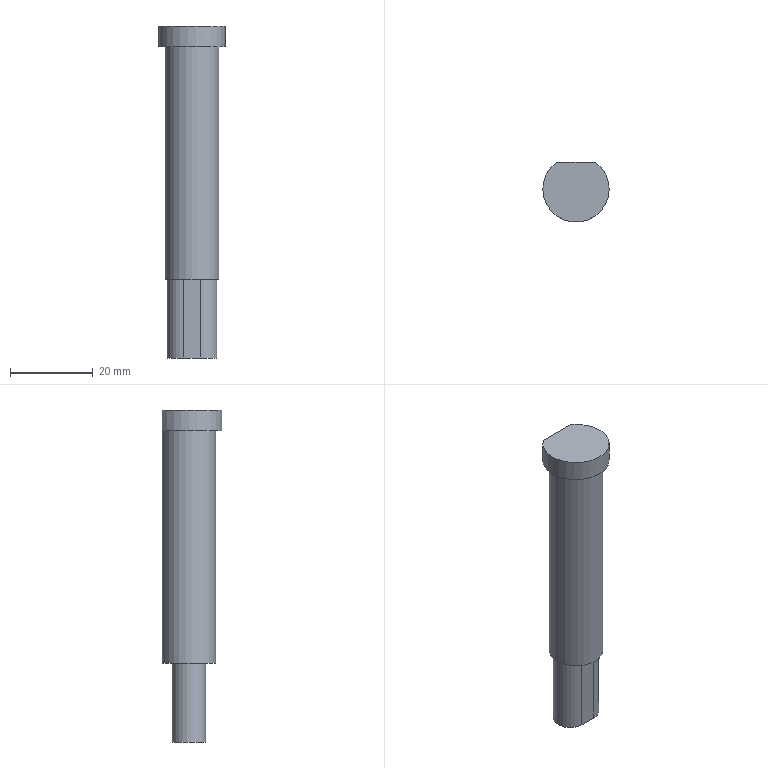Part | NX | features solid 2 | 1 solid | 11 faces | box 16 x 14.5 x 80 mm | volume 9985 mm3 | plane 7 | cylinder 4 | commonest cylinder face diameters 8.1 x2 13 x1 16 x1
STEP:
#1=CARTESIAN_POINT('',(-1262.413,378.428,72.));
#2=VERTEX_POINT('',#1);
#3=CARTESIAN_POINT('',(-1262.413,384.928,72.));
#4=DIRECTION('',(0.,0.,1.));
#5=DIRECTION('',(0.,-1.,0.));
#6=AXIS2_PLACEMENT_3D('',#3,#4,#5);
#7=CIRCLE('',#6,6.5);
#8=EDGE_CURVE('',#2,#2,#7,.T.);
#9=ORIENTED_EDGE('',*,*,#8,.F.);
#10=EDGE_LOOP('',(#9));
#11=FACE_BOUND('',#10,.T.);
#12=CARTESIAN_POINT('',(-1260.413,380.878,72.));
#13=VERTEX_POINT('',#12);
#14=CARTESIAN_POINT('',(-1264.413,380.878,72.));
#15=VERTEX_POINT('',#14);
#16=CARTESIAN_POINT('',(-1262.413,380.878,72.));
#17=DIRECTION('',(-1.,0.,0.));
#18=VECTOR('',#17,1000.);
#19=LINE('',#16,#18);
#20=EDGE_CURVE('',#13,#15,#19,.T.);
#21=ORIENTED_EDGE('',*,*,#20,.F.);
#22=CARTESIAN_POINT('',(-1260.413,388.978,72.));
#23=VERTEX_POINT('',#22);
#24=CARTESIAN_POINT('',(-1260.413,384.928,72.));
#25=DIRECTION('',(0.,0.,1.));
#26=DIRECTION('',(0.,-1.,0.));
#27=AXIS2_PLACEMENT_3D('',#24,#25,#26);
#28=CIRCLE('',#27,4.05);
#29=EDGE_CURVE('',#13,#23,#28,.T.);
#30=ORIENTED_EDGE('',*,*,#29,.T.);
#31=CARTESIAN_POINT('',(-1264.413,388.978,72.));
#32=VERTEX_POINT('',#31);
#33=CARTESIAN_POINT('',(-1262.413,388.978,72.));
#34=DIRECTION('',(-1.,0.,0.));
#35=VECTOR('',#34,1000.);
#36=LINE('',#33,#35);
#37=EDGE_CURVE('',#23,#32,#36,.T.);
#38=ORIENTED_EDGE('',*,*,#37,.T.);
#39=CARTESIAN_POINT('',(-1264.413,384.928,72.));
#40=DIRECTION('',(0.,0.,1.));
#41=DIRECTION('',(0.,-1.,0.));
#42=AXIS2_PLACEMENT_3D('',#39,#40,#41);
#43=CIRCLE('',#42,4.05);
#44=EDGE_CURVE('',#32,#15,#43,.T.);
#45=ORIENTED_EDGE('',*,*,#44,.T.);
#46=EDGE_LOOP('',(#21,#30,#38,#45));
#47=FACE_BOUND('',#46,.T.);
#48=CARTESIAN_POINT('',(-1262.413,384.928,72.));
#49=DIRECTION('',(0.,0.,1.));
#50=DIRECTION('',(0.,-1.,0.));
#51=AXIS2_PLACEMENT_3D('',#48,#49,#50);
#52=PLANE('',#51);
#53=ADVANCED_FACE('',(#11,#47),#52,.F.);
#54=ORIENTED_EDGE('',*,*,#8,.T.);
#55=EDGE_LOOP('',(#54));
#56=FACE_BOUND('',#55,.T.);
#57=CARTESIAN_POINT('',(-1262.413,391.428,128.));
#58=VERTEX_POINT('',#57);
#59=CARTESIAN_POINT('',(-1262.413,384.928,128.));
#60=DIRECTION('',(0.,0.,1.));
#61=DIRECTION('',(0.,-1.,0.));
#62=AXIS2_PLACEMENT_3D('',#59,#60,#61);
#63=CIRCLE('',#62,6.5);
#64=EDGE_CURVE('',#58,#58,#63,.T.);
#65=ORIENTED_EDGE('',*,*,#64,.F.);
#66=EDGE_LOOP('',(#65));
#67=FACE_BOUND('',#66,.T.);
#68=CARTESIAN_POINT('',(-1262.413,384.928,133.));
#69=DIRECTION('',(0.,0.,-1.));
#70=DIRECTION('',(0.,1.,0.));
#71=AXIS2_PLACEMENT_3D('',#68,#69,#70);
#72=CYLINDRICAL_SURFACE('',#71,6.5);
#73=ADVANCED_FACE('',(#56,#67),#72,.T.);
#74=CARTESIAN_POINT('',(-1267.077,391.428,128.));
#75=VERTEX_POINT('',#74);
#76=CARTESIAN_POINT('',(-1257.75,391.428,128.));
#77=VERTEX_POINT('',#76);
#78=CARTESIAN_POINT('',(-1262.413,384.928,128.));
#79=DIRECTION('',(0.,0.,1.));
#80=DIRECTION('',(0.,-1.,0.));
#81=AXIS2_PLACEMENT_3D('',#78,#79,#80);
#82=CIRCLE('',#81,8.);
#83=EDGE_CURVE('',#75,#77,#82,.T.);
#84=ORIENTED_EDGE('',*,*,#83,.F.);
#85=CARTESIAN_POINT('',(-1262.413,391.428,128.));
#86=DIRECTION('',(1.,0.,0.));
#87=VECTOR('',#86,1000.);
#88=LINE('',#85,#87);
#89=EDGE_CURVE('',#75,#58,#88,.T.);
#90=ORIENTED_EDGE('',*,*,#89,.T.);
#91=ORIENTED_EDGE('',*,*,#64,.T.);
#92=CARTESIAN_POINT('',(-1262.413,391.428,128.));
#93=DIRECTION('',(1.,0.,0.));
#94=VECTOR('',#93,1000.);
#95=LINE('',#92,#94);
#96=EDGE_CURVE('',#58,#77,#95,.T.);
#97=ORIENTED_EDGE('',*,*,#96,.T.);
#98=EDGE_LOOP('',(#84,#90,#91,#97));
#99=FACE_BOUND('',#98,.T.);
#100=CARTESIAN_POINT('',(-1262.413,384.928,128.));
#101=DIRECTION('',(0.,0.,1.));
#102=DIRECTION('',(0.,-1.,0.));
#103=AXIS2_PLACEMENT_3D('',#100,#101,#102);
#104=PLANE('',#103);
#105=ADVANCED_FACE('',(#99),#104,.F.);
#106=CARTESIAN_POINT('',(-1257.75,391.428,133.));
#107=VERTEX_POINT('',#106);
#108=CARTESIAN_POINT('',(-1257.75,391.428,137.));
#109=DIRECTION('',(0.,0.,-1.));
#110=VECTOR('',#109,1000.);
#111=LINE('',#108,#110);
#112=EDGE_CURVE('',#107,#77,#111,.T.);
#113=ORIENTED_EDGE('',*,*,#112,.F.);
#114=CARTESIAN_POINT('',(-1267.077,391.428,133.));
#115=VERTEX_POINT('',#114);
#116=CARTESIAN_POINT('',(-1262.413,384.928,133.));
#117=DIRECTION('',(0.,0.,1.));
#118=DIRECTION('',(0.,-1.,0.));
#119=AXIS2_PLACEMENT_3D('',#116,#117,#118);
#120=CIRCLE('',#119,8.);
#121=EDGE_CURVE('',#115,#107,#120,.T.);
#122=ORIENTED_EDGE('',*,*,#121,.F.);
#123=CARTESIAN_POINT('',(-1267.077,391.428,137.));
#124=DIRECTION('',(0.,0.,-1.));
#125=VECTOR('',#124,1000.);
#126=LINE('',#123,#125);
#127=EDGE_CURVE('',#75,#115,#126,.F.);
#128=ORIENTED_EDGE('',*,*,#127,.F.);
#129=ORIENTED_EDGE('',*,*,#83,.T.);
#130=EDGE_LOOP('',(#113,#122,#128,#129));
#131=FACE_BOUND('',#130,.T.);
#132=CARTESIAN_POINT('',(-1262.413,384.928,128.));
#133=DIRECTION('',(0.,0.,1.));
#134=DIRECTION('',(0.,-1.,0.));
#135=AXIS2_PLACEMENT_3D('',#132,#133,#134);
#136=CYLINDRICAL_SURFACE('',#135,8.);
#137=ADVANCED_FACE('',(#131),#136,.T.);
#138=CARTESIAN_POINT('',(-1262.413,391.428,133.));
#139=DIRECTION('',(1.,0.,0.));
#140=VECTOR('',#139,1000.);
#141=LINE('',#138,#140);
#142=EDGE_CURVE('',#115,#107,#141,.T.);
#143=ORIENTED_EDGE('',*,*,#142,.F.);
#144=ORIENTED_EDGE('',*,*,#121,.T.);
#145=EDGE_LOOP('',(#143,#144));
#146=FACE_BOUND('',#145,.T.);
#147=CARTESIAN_POINT('',(-1262.413,384.928,133.));
#148=DIRECTION('',(0.,0.,1.));
#149=DIRECTION('',(0.,-1.,0.));
#150=AXIS2_PLACEMENT_3D('',#147,#148,#149);
#151=PLANE('',#150);
#152=ADVANCED_FACE('',(#146),#151,.T.);
#153=ORIENTED_EDGE('',*,*,#127,.T.);
#154=ORIENTED_EDGE('',*,*,#142,.T.);
#155=ORIENTED_EDGE('',*,*,#112,.T.);
#156=ORIENTED_EDGE('',*,*,#96,.F.);
#157=ORIENTED_EDGE('',*,*,#89,.F.);
#158=EDGE_LOOP('',(#153,#154,#155,#156,#157));
#159=FACE_BOUND('',#158,.T.);
#160=CARTESIAN_POINT('',(-1257.75,391.428,137.));
#161=DIRECTION('',(0.,-1.,0.));
#162=DIRECTION('',(0.,0.,-1.));
#163=AXIS2_PLACEMENT_3D('',#160,#161,#162);
#164=PLANE('',#163);
#165=ADVANCED_FACE('',(#159),#164,.F.);
#166=CARTESIAN_POINT('',(-1260.413,380.878,53.));
#167=VERTEX_POINT('',#166);
#168=CARTESIAN_POINT('',(-1260.413,380.878,53.));
#169=DIRECTION('',(0.,0.,1.));
#170=VECTOR('',#169,1000.);
#171=LINE('',#168,#170);
#172=EDGE_CURVE('',#167,#13,#171,.T.);
#173=ORIENTED_EDGE('',*,*,#172,.T.);
#174=ORIENTED_EDGE('',*,*,#20,.T.);
#175=CARTESIAN_POINT('',(-1264.413,380.878,53.));
#176=VERTEX_POINT('',#175);
#177=CARTESIAN_POINT('',(-1264.413,380.878,53.));
#178=DIRECTION('',(0.,0.,1.));
#179=VECTOR('',#178,1000.);
#180=LINE('',#177,#179);
#181=EDGE_CURVE('',#176,#15,#180,.T.);
#182=ORIENTED_EDGE('',*,*,#181,.F.);
#183=CARTESIAN_POINT('',(-1260.413,380.878,53.));
#184=DIRECTION('',(-1.,0.,0.));
#185=VECTOR('',#184,1000.);
#186=LINE('',#183,#185);
#187=EDGE_CURVE('',#167,#176,#186,.T.);
#188=ORIENTED_EDGE('',*,*,#187,.F.);
#189=EDGE_LOOP('',(#173,#174,#182,#188));
#190=FACE_BOUND('',#189,.T.);
#191=CARTESIAN_POINT('',(-1260.413,380.878,53.));
#192=DIRECTION('',(0.,1.,0.));
#193=DIRECTION('',(0.,0.,1.));
#194=AXIS2_PLACEMENT_3D('',#191,#192,#193);
#195=PLANE('',#194);
#196=ADVANCED_FACE('',(#190),#195,.F.);
#197=ORIENTED_EDGE('',*,*,#44,.F.);
#198=CARTESIAN_POINT('',(-1264.413,388.978,53.));
#199=VERTEX_POINT('',#198);
#200=CARTESIAN_POINT('',(-1264.413,388.978,53.));
#201=DIRECTION('',(0.,0.,1.));
#202=VECTOR('',#201,1000.);
#203=LINE('',#200,#202);
#204=EDGE_CURVE('',#199,#32,#203,.T.);
#205=ORIENTED_EDGE('',*,*,#204,.F.);
#206=CARTESIAN_POINT('',(-1264.413,384.928,53.));
#207=DIRECTION('',(0.,0.,1.));
#208=DIRECTION('',(0.,-1.,0.));
#209=AXIS2_PLACEMENT_3D('',#206,#207,#208);
#210=CIRCLE('',#209,4.05);
#211=EDGE_CURVE('',#199,#176,#210,.T.);
#212=ORIENTED_EDGE('',*,*,#211,.T.);
#213=ORIENTED_EDGE('',*,*,#181,.T.);
#214=EDGE_LOOP('',(#197,#205,#212,#213));
#215=FACE_BOUND('',#214,.T.);
#216=CARTESIAN_POINT('',(-1264.413,384.928,53.));
#217=DIRECTION('',(0.,0.,1.));
#218=DIRECTION('',(0.,-1.,0.));
#219=AXIS2_PLACEMENT_3D('',#216,#217,#218);
#220=CYLINDRICAL_SURFACE('',#219,4.05);
#221=ADVANCED_FACE('',(#215),#220,.T.);
#222=ORIENTED_EDGE('',*,*,#37,.F.);
#223=CARTESIAN_POINT('',(-1260.413,388.978,53.));
#224=VERTEX_POINT('',#223);
#225=CARTESIAN_POINT('',(-1260.413,388.978,53.));
#226=DIRECTION('',(0.,0.,1.));
#227=VECTOR('',#226,1000.);
#228=LINE('',#225,#227);
#229=EDGE_CURVE('',#224,#23,#228,.T.);
#230=ORIENTED_EDGE('',*,*,#229,.F.);
#231=CARTESIAN_POINT('',(-1260.413,388.978,53.));
#232=DIRECTION('',(-1.,0.,0.));
#233=VECTOR('',#232,1000.);
#234=LINE('',#231,#233);
#235=EDGE_CURVE('',#224,#199,#234,.T.);
#236=ORIENTED_EDGE('',*,*,#235,.T.);
#237=ORIENTED_EDGE('',*,*,#204,.T.);
#238=EDGE_LOOP('',(#222,#230,#236,#237));
#239=FACE_BOUND('',#238,.T.);
#240=CARTESIAN_POINT('',(-1260.413,388.978,53.));
#241=DIRECTION('',(0.,1.,0.));
#242=DIRECTION('',(0.,0.,1.));
#243=AXIS2_PLACEMENT_3D('',#240,#241,#242);
#244=PLANE('',#243);
#245=ADVANCED_FACE('',(#239),#244,.T.);
#246=ORIENTED_EDGE('',*,*,#29,.F.);
#247=ORIENTED_EDGE('',*,*,#172,.F.);
#248=CARTESIAN_POINT('',(-1260.413,384.928,53.));
#249=DIRECTION('',(0.,0.,1.));
#250=DIRECTION('',(0.,-1.,0.));
#251=AXIS2_PLACEMENT_3D('',#248,#249,#250);
#252=CIRCLE('',#251,4.05);
#253=EDGE_CURVE('',#167,#224,#252,.T.);
#254=ORIENTED_EDGE('',*,*,#253,.T.);
#255=ORIENTED_EDGE('',*,*,#229,.T.);
#256=EDGE_LOOP('',(#246,#247,#254,#255));
#257=FACE_BOUND('',#256,.T.);
#258=CARTESIAN_POINT('',(-1260.413,384.928,53.));
#259=DIRECTION('',(0.,0.,1.));
#260=DIRECTION('',(0.,-1.,0.));
#261=AXIS2_PLACEMENT_3D('',#258,#259,#260);
#262=CYLINDRICAL_SURFACE('',#261,4.05);
#263=ADVANCED_FACE('',(#257),#262,.T.);
#264=ORIENTED_EDGE('',*,*,#187,.T.);
#265=ORIENTED_EDGE('',*,*,#211,.F.);
#266=ORIENTED_EDGE('',*,*,#235,.F.);
#267=ORIENTED_EDGE('',*,*,#253,.F.);
#268=EDGE_LOOP('',(#264,#265,#266,#267));
#269=FACE_BOUND('',#268,.T.);
#270=CARTESIAN_POINT('',(-1264.413,384.928,53.));
#271=DIRECTION('',(0.,0.,1.));
#272=DIRECTION('',(0.,-1.,0.));
#273=AXIS2_PLACEMENT_3D('',#270,#271,#272);
#274=PLANE('',#273);
#275=ADVANCED_FACE('',(#269),#274,.F.);
#276=CLOSED_SHELL('',(#53,#73,#105,#137,#152,#165,#196,#221,#245,#263,#275));
#277=MANIFOLD_SOLID_BREP('',#276);
#278=(LENGTH_UNIT()NAMED_UNIT(*)SI_UNIT(.MILLI.,.METRE.));
#279=UNCERTAINTY_MEASURE_WITH_UNIT(LENGTH_MEASURE(0.00001),#278,'','');
#280=(NAMED_UNIT(*)PLANE_ANGLE_UNIT()SI_UNIT($,.RADIAN.));
#281=(NAMED_UNIT(*)SI_UNIT($,.STERADIAN.)SOLID_ANGLE_UNIT());
#282=(GEOMETRIC_REPRESENTATION_CONTEXT(3)GLOBAL_UNCERTAINTY_ASSIGNED_CONTEXT((#279))GLOBAL_UNIT_ASSIGNED_CONTEXT((#278,#280,#281))REPRESENTATION_CONTEXT('',''));
#283=ADVANCED_BREP_SHAPE_REPRESENTATION('',(#277),#282);